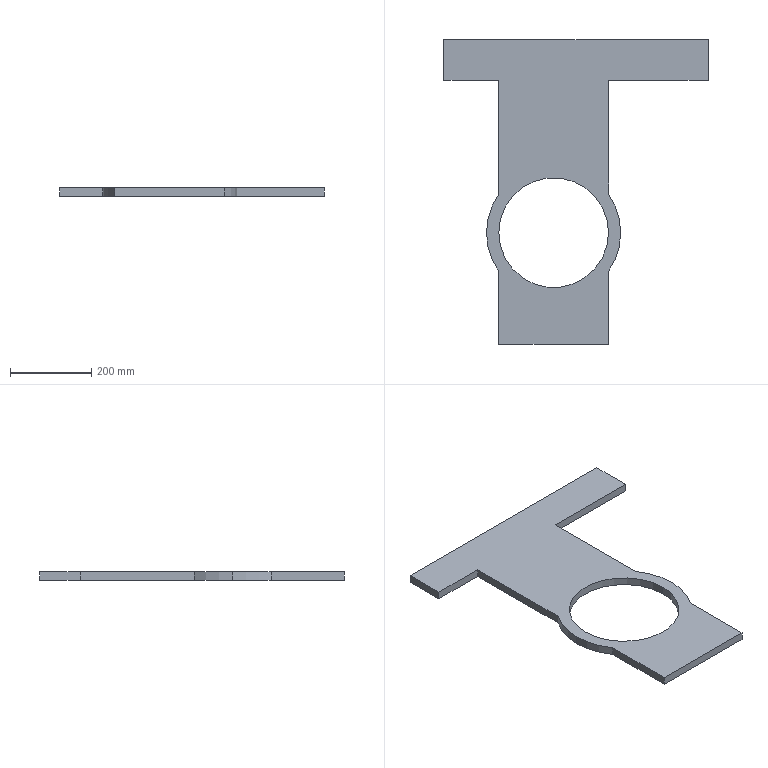Part | SolidWorks | features ICE 2, Extrusion 1 | 1 solid | 17 faces | box 650 x 750 x 20 mm | volume 3819673 mm3 | plane 12 | cylinder 5 | commonest cylinder face diameters 330 x3 270 x2
STEP:
#1=CARTESIAN_POINT('',(-135.,0.,20.));
#2=VERTEX_POINT('',#1);
#3=CARTESIAN_POINT('',(135.,0.,20.));
#4=VERTEX_POINT('',#3);
#5=CARTESIAN_POINT('',(0.,0.,20.));
#6=DIRECTION('',(0.,0.,1.));
#7=DIRECTION('',(1.,0.,0.));
#8=AXIS2_PLACEMENT_3D('',#5,#6,#7);
#9=CIRCLE('',#8,135.);
#10=EDGE_CURVE('',#2,#4,#9,.T.);
#11=ORIENTED_EDGE('',*,*,#10,.T.);
#12=CARTESIAN_POINT('',(135.,0.,0.));
#13=VERTEX_POINT('',#12);
#14=CARTESIAN_POINT('',(135.,0.,20.));
#15=DIRECTION('',(0.,0.,-1.));
#16=VECTOR('',#15,1000.);
#17=LINE('',#14,#16);
#18=EDGE_CURVE('',#4,#13,#17,.T.);
#19=ORIENTED_EDGE('',*,*,#18,.T.);
#20=CARTESIAN_POINT('',(-135.,0.,0.));
#21=VERTEX_POINT('',#20);
#22=CARTESIAN_POINT('',(0.,0.,0.));
#23=DIRECTION('',(0.,0.,1.));
#24=DIRECTION('',(1.,0.,0.));
#25=AXIS2_PLACEMENT_3D('',#22,#23,#24);
#26=CIRCLE('',#25,135.);
#27=EDGE_CURVE('',#21,#13,#26,.T.);
#28=ORIENTED_EDGE('',*,*,#27,.F.);
#29=CARTESIAN_POINT('',(-135.,0.,20.));
#30=DIRECTION('',(0.,0.,-1.));
#31=VECTOR('',#30,1000.);
#32=LINE('',#29,#31);
#33=EDGE_CURVE('',#2,#21,#32,.T.);
#34=ORIENTED_EDGE('',*,*,#33,.F.);
#35=EDGE_LOOP('',(#11,#19,#28,#34));
#36=FACE_OUTER_BOUND('',#35,.T.);
#37=CARTESIAN_POINT('',(0.,0.,20.));
#38=DIRECTION('',(0.,0.,-1.));
#39=DIRECTION('',(-1.,0.,0.));
#40=AXIS2_PLACEMENT_3D('',#37,#38,#39);
#41=CYLINDRICAL_SURFACE('',#40,135.);
#42=ADVANCED_FACE('',(#36),#41,.F.);
#43=CARTESIAN_POINT('',(-165.,0.,20.));
#44=VERTEX_POINT('',#43);
#45=CARTESIAN_POINT('',(-135.,-94.868,20.));
#46=VERTEX_POINT('',#45);
#47=CARTESIAN_POINT('',(0.,0.,20.));
#48=DIRECTION('',(0.,0.,1.));
#49=DIRECTION('',(1.,0.,0.));
#50=AXIS2_PLACEMENT_3D('',#47,#48,#49);
#51=CIRCLE('',#50,165.);
#52=EDGE_CURVE('',#44,#46,#51,.T.);
#53=ORIENTED_EDGE('',*,*,#52,.F.);
#54=CARTESIAN_POINT('',(-165.,0.,0.));
#55=VERTEX_POINT('',#54);
#56=CARTESIAN_POINT('',(-165.,0.,20.));
#57=DIRECTION('',(0.,0.,-1.));
#58=VECTOR('',#57,1000.);
#59=LINE('',#56,#58);
#60=EDGE_CURVE('',#44,#55,#59,.T.);
#61=ORIENTED_EDGE('',*,*,#60,.T.);
#62=CARTESIAN_POINT('',(-135.,-94.868,0.));
#63=VERTEX_POINT('',#62);
#64=CARTESIAN_POINT('',(0.,0.,0.));
#65=DIRECTION('',(0.,0.,1.));
#66=DIRECTION('',(1.,0.,0.));
#67=AXIS2_PLACEMENT_3D('',#64,#65,#66);
#68=CIRCLE('',#67,165.);
#69=EDGE_CURVE('',#55,#63,#68,.T.);
#70=ORIENTED_EDGE('',*,*,#69,.T.);
#71=CARTESIAN_POINT('',(-135.,-94.868,20.));
#72=DIRECTION('',(0.,0.,-1.));
#73=VECTOR('',#72,1000.);
#74=LINE('',#71,#73);
#75=EDGE_CURVE('',#46,#63,#74,.T.);
#76=ORIENTED_EDGE('',*,*,#75,.F.);
#77=EDGE_LOOP('',(#53,#61,#70,#76));
#78=FACE_OUTER_BOUND('',#77,.T.);
#79=CARTESIAN_POINT('',(0.,0.,20.));
#80=DIRECTION('',(0.,0.,-1.));
#81=DIRECTION('',(-1.,0.,0.));
#82=AXIS2_PLACEMENT_3D('',#79,#80,#81);
#83=CYLINDRICAL_SURFACE('',#82,165.);
#84=ADVANCED_FACE('',(#78),#83,.T.);
#85=CARTESIAN_POINT('',(135.,375.,20.));
#86=VERTEX_POINT('',#85);
#87=CARTESIAN_POINT('',(135.,375.,0.));
#88=VERTEX_POINT('',#87);
#89=CARTESIAN_POINT('',(135.,375.,20.));
#90=DIRECTION('',(0.,0.,-1.));
#91=VECTOR('',#90,1000.);
#92=LINE('',#89,#91);
#93=EDGE_CURVE('',#86,#88,#92,.T.);
#94=ORIENTED_EDGE('',*,*,#93,.F.);
#95=CARTESIAN_POINT('',(135.,94.868,20.));
#96=VERTEX_POINT('',#95);
#97=CARTESIAN_POINT('',(135.,475.,20.));
#98=DIRECTION('',(0.,1.,0.));
#99=VECTOR('',#98,1000.);
#100=LINE('',#97,#99);
#101=EDGE_CURVE('',#96,#86,#100,.T.);
#102=ORIENTED_EDGE('',*,*,#101,.F.);
#103=CARTESIAN_POINT('',(135.,94.868,0.));
#104=VERTEX_POINT('',#103);
#105=CARTESIAN_POINT('',(135.,94.868,20.));
#106=DIRECTION('',(0.,0.,-1.));
#107=VECTOR('',#106,1000.);
#108=LINE('',#105,#107);
#109=EDGE_CURVE('',#96,#104,#108,.T.);
#110=ORIENTED_EDGE('',*,*,#109,.T.);
#111=CARTESIAN_POINT('',(135.,475.,0.));
#112=DIRECTION('',(0.,1.,0.));
#113=VECTOR('',#112,1000.);
#114=LINE('',#111,#113);
#115=EDGE_CURVE('',#104,#88,#114,.T.);
#116=ORIENTED_EDGE('',*,*,#115,.T.);
#117=EDGE_LOOP('',(#94,#102,#110,#116));
#118=FACE_OUTER_BOUND('',#117,.T.);
#119=CARTESIAN_POINT('',(135.,475.,20.));
#120=DIRECTION('',(-1.,0.,0.));
#121=DIRECTION('',(0.,-1.,0.));
#122=AXIS2_PLACEMENT_3D('',#119,#120,#121);
#123=PLANE('',#122);
#124=ADVANCED_FACE('',(#118),#123,.F.);
#125=CARTESIAN_POINT('',(135.,-275.,20.));
#126=VERTEX_POINT('',#125);
#127=CARTESIAN_POINT('',(-135.,-275.,20.));
#128=VERTEX_POINT('',#127);
#129=CARTESIAN_POINT('',(135.,-275.,20.));
#130=DIRECTION('',(-1.,0.,0.));
#131=VECTOR('',#130,1000.);
#132=LINE('',#129,#131);
#133=EDGE_CURVE('',#126,#128,#132,.T.);
#134=ORIENTED_EDGE('',*,*,#133,.F.);
#135=CARTESIAN_POINT('',(135.,-94.868,20.));
#136=VERTEX_POINT('',#135);
#137=CARTESIAN_POINT('',(135.,-475.,20.));
#138=DIRECTION('',(0.,1.,0.));
#139=VECTOR('',#138,1000.);
#140=LINE('',#137,#139);
#141=EDGE_CURVE('',#126,#136,#140,.T.);
#142=ORIENTED_EDGE('',*,*,#141,.T.);
#143=CARTESIAN_POINT('',(0.,0.,20.));
#144=DIRECTION('',(0.,0.,1.));
#145=DIRECTION('',(1.,0.,0.));
#146=AXIS2_PLACEMENT_3D('',#143,#144,#145);
#147=CIRCLE('',#146,165.);
#148=EDGE_CURVE('',#136,#96,#147,.T.);
#149=ORIENTED_EDGE('',*,*,#148,.T.);
#150=ORIENTED_EDGE('',*,*,#101,.T.);
#151=CARTESIAN_POINT('',(380.,375.,20.));
#152=VERTEX_POINT('',#151);
#153=CARTESIAN_POINT('',(0.,375.,20.));
#154=DIRECTION('',(1.,0.,0.));
#155=VECTOR('',#154,1000.);
#156=LINE('',#153,#155);
#157=EDGE_CURVE('',#86,#152,#156,.T.);
#158=ORIENTED_EDGE('',*,*,#157,.T.);
#159=CARTESIAN_POINT('',(380.,475.,20.));
#160=VERTEX_POINT('',#159);
#161=CARTESIAN_POINT('',(380.,0.,20.));
#162=DIRECTION('',(0.,-1.,0.));
#163=VECTOR('',#162,1000.);
#164=LINE('',#161,#163);
#165=EDGE_CURVE('',#160,#152,#164,.T.);
#166=ORIENTED_EDGE('',*,*,#165,.F.);
#167=CARTESIAN_POINT('',(-270.,475.,20.));
#168=VERTEX_POINT('',#167);
#169=CARTESIAN_POINT('',(135.,475.,20.));
#170=DIRECTION('',(-1.,0.,0.));
#171=VECTOR('',#170,1000.);
#172=LINE('',#169,#171);
#173=EDGE_CURVE('',#160,#168,#172,.T.);
#174=ORIENTED_EDGE('',*,*,#173,.T.);
#175=CARTESIAN_POINT('',(-270.,375.,20.));
#176=VERTEX_POINT('',#175);
#177=CARTESIAN_POINT('',(-270.,0.,20.));
#178=DIRECTION('',(0.,-1.,0.));
#179=VECTOR('',#178,1000.);
#180=LINE('',#177,#179);
#181=EDGE_CURVE('',#168,#176,#180,.T.);
#182=ORIENTED_EDGE('',*,*,#181,.T.);
#183=CARTESIAN_POINT('',(-135.,375.,20.));
#184=VERTEX_POINT('',#183);
#185=CARTESIAN_POINT('',(0.,375.,20.));
#186=DIRECTION('',(-1.,0.,0.));
#187=VECTOR('',#186,1000.);
#188=LINE('',#185,#187);
#189=EDGE_CURVE('',#184,#176,#188,.T.);
#190=ORIENTED_EDGE('',*,*,#189,.F.);
#191=CARTESIAN_POINT('',(-135.,94.868,20.));
#192=VERTEX_POINT('',#191);
#193=CARTESIAN_POINT('',(-135.,475.,20.));
#194=DIRECTION('',(0.,-1.,0.));
#195=VECTOR('',#194,1000.);
#196=LINE('',#193,#195);
#197=EDGE_CURVE('',#184,#192,#196,.T.);
#198=ORIENTED_EDGE('',*,*,#197,.T.);
#199=CARTESIAN_POINT('',(0.,0.,20.));
#200=DIRECTION('',(0.,0.,1.));
#201=DIRECTION('',(1.,0.,0.));
#202=AXIS2_PLACEMENT_3D('',#199,#200,#201);
#203=CIRCLE('',#202,165.);
#204=EDGE_CURVE('',#192,#44,#203,.T.);
#205=ORIENTED_EDGE('',*,*,#204,.T.);
#206=ORIENTED_EDGE('',*,*,#52,.T.);
#207=CARTESIAN_POINT('',(-135.,-475.,20.));
#208=DIRECTION('',(0.,-1.,0.));
#209=VECTOR('',#208,1000.);
#210=LINE('',#207,#209);
#211=EDGE_CURVE('',#46,#128,#210,.T.);
#212=ORIENTED_EDGE('',*,*,#211,.T.);
#213=EDGE_LOOP('',(#134,#142,#149,#150,#158,#166,#174,#182,#190,#198,#205,#206,#212));
#214=FACE_OUTER_BOUND('',#213,.T.);
#215=ORIENTED_EDGE('',*,*,#10,.F.);
#216=CARTESIAN_POINT('',(0.,0.,20.));
#217=DIRECTION('',(0.,0.,1.));
#218=DIRECTION('',(1.,0.,0.));
#219=AXIS2_PLACEMENT_3D('',#216,#217,#218);
#220=CIRCLE('',#219,135.);
#221=EDGE_CURVE('',#4,#2,#220,.T.);
#222=ORIENTED_EDGE('',*,*,#221,.F.);
#223=EDGE_LOOP('',(#215,#222));
#224=FACE_BOUND('',#223,.T.);
#225=CARTESIAN_POINT('',(0.,0.,20.));
#226=DIRECTION('',(0.,0.,1.));
#227=DIRECTION('',(1.,0.,0.));
#228=AXIS2_PLACEMENT_3D('',#225,#226,#227);
#229=PLANE('',#228);
#230=ADVANCED_FACE('',(#214,#224),#229,.T.);
#231=CARTESIAN_POINT('',(135.,-275.,0.));
#232=VERTEX_POINT('',#231);
#233=CARTESIAN_POINT('',(135.,-94.868,0.));
#234=VERTEX_POINT('',#233);
#235=CARTESIAN_POINT('',(135.,-475.,0.));
#236=DIRECTION('',(0.,1.,0.));
#237=VECTOR('',#236,1000.);
#238=LINE('',#235,#237);
#239=EDGE_CURVE('',#232,#234,#238,.T.);
#240=ORIENTED_EDGE('',*,*,#239,.F.);
#241=CARTESIAN_POINT('',(-135.,-275.,0.));
#242=VERTEX_POINT('',#241);
#243=CARTESIAN_POINT('',(135.,-275.,0.));
#244=DIRECTION('',(-1.,0.,0.));
#245=VECTOR('',#244,1000.);
#246=LINE('',#243,#245);
#247=EDGE_CURVE('',#232,#242,#246,.T.);
#248=ORIENTED_EDGE('',*,*,#247,.T.);
#249=CARTESIAN_POINT('',(-135.,-475.,0.));
#250=DIRECTION('',(0.,-1.,0.));
#251=VECTOR('',#250,1000.);
#252=LINE('',#249,#251);
#253=EDGE_CURVE('',#63,#242,#252,.T.);
#254=ORIENTED_EDGE('',*,*,#253,.F.);
#255=ORIENTED_EDGE('',*,*,#69,.F.);
#256=CARTESIAN_POINT('',(-135.,94.868,0.));
#257=VERTEX_POINT('',#256);
#258=CARTESIAN_POINT('',(0.,0.,0.));
#259=DIRECTION('',(0.,0.,1.));
#260=DIRECTION('',(1.,0.,0.));
#261=AXIS2_PLACEMENT_3D('',#258,#259,#260);
#262=CIRCLE('',#261,165.);
#263=EDGE_CURVE('',#257,#55,#262,.T.);
#264=ORIENTED_EDGE('',*,*,#263,.F.);
#265=CARTESIAN_POINT('',(-135.,375.,0.));
#266=VERTEX_POINT('',#265);
#267=CARTESIAN_POINT('',(-135.,475.,0.));
#268=DIRECTION('',(0.,-1.,0.));
#269=VECTOR('',#268,1000.);
#270=LINE('',#267,#269);
#271=EDGE_CURVE('',#266,#257,#270,.T.);
#272=ORIENTED_EDGE('',*,*,#271,.F.);
#273=CARTESIAN_POINT('',(-270.,375.,0.));
#274=VERTEX_POINT('',#273);
#275=CARTESIAN_POINT('',(0.,375.,0.));
#276=DIRECTION('',(-1.,0.,0.));
#277=VECTOR('',#276,1000.);
#278=LINE('',#275,#277);
#279=EDGE_CURVE('',#266,#274,#278,.T.);
#280=ORIENTED_EDGE('',*,*,#279,.T.);
#281=CARTESIAN_POINT('',(-270.,475.,0.));
#282=VERTEX_POINT('',#281);
#283=CARTESIAN_POINT('',(-270.,0.,0.));
#284=DIRECTION('',(0.,-1.,0.));
#285=VECTOR('',#284,1000.);
#286=LINE('',#283,#285);
#287=EDGE_CURVE('',#282,#274,#286,.T.);
#288=ORIENTED_EDGE('',*,*,#287,.F.);
#289=CARTESIAN_POINT('',(380.,475.,0.));
#290=VERTEX_POINT('',#289);
#291=CARTESIAN_POINT('',(135.,475.,0.));
#292=DIRECTION('',(-1.,0.,0.));
#293=VECTOR('',#292,1000.);
#294=LINE('',#291,#293);
#295=EDGE_CURVE('',#290,#282,#294,.T.);
#296=ORIENTED_EDGE('',*,*,#295,.F.);
#297=CARTESIAN_POINT('',(380.,375.,0.));
#298=VERTEX_POINT('',#297);
#299=CARTESIAN_POINT('',(380.,0.,0.));
#300=DIRECTION('',(0.,-1.,0.));
#301=VECTOR('',#300,1000.);
#302=LINE('',#299,#301);
#303=EDGE_CURVE('',#290,#298,#302,.T.);
#304=ORIENTED_EDGE('',*,*,#303,.T.);
#305=CARTESIAN_POINT('',(0.,375.,0.));
#306=DIRECTION('',(1.,0.,0.));
#307=VECTOR('',#306,1000.);
#308=LINE('',#305,#307);
#309=EDGE_CURVE('',#88,#298,#308,.T.);
#310=ORIENTED_EDGE('',*,*,#309,.F.);
#311=ORIENTED_EDGE('',*,*,#115,.F.);
#312=CARTESIAN_POINT('',(0.,0.,0.));
#313=DIRECTION('',(0.,0.,1.));
#314=DIRECTION('',(1.,0.,0.));
#315=AXIS2_PLACEMENT_3D('',#312,#313,#314);
#316=CIRCLE('',#315,165.);
#317=EDGE_CURVE('',#234,#104,#316,.T.);
#318=ORIENTED_EDGE('',*,*,#317,.F.);
#319=EDGE_LOOP('',(#240,#248,#254,#255,#264,#272,#280,#288,#296,#304,#310,#311,#318));
#320=FACE_OUTER_BOUND('',#319,.T.);
#321=ORIENTED_EDGE('',*,*,#27,.T.);
#322=CARTESIAN_POINT('',(0.,0.,0.));
#323=DIRECTION('',(0.,0.,1.));
#324=DIRECTION('',(1.,0.,0.));
#325=AXIS2_PLACEMENT_3D('',#322,#323,#324);
#326=CIRCLE('',#325,135.);
#327=EDGE_CURVE('',#13,#21,#326,.T.);
#328=ORIENTED_EDGE('',*,*,#327,.T.);
#329=EDGE_LOOP('',(#321,#328));
#330=FACE_BOUND('',#329,.T.);
#331=CARTESIAN_POINT('',(0.,0.,0.));
#332=DIRECTION('',(0.,0.,1.));
#333=DIRECTION('',(1.,0.,0.));
#334=AXIS2_PLACEMENT_3D('',#331,#332,#333);
#335=PLANE('',#334);
#336=ADVANCED_FACE('',(#320,#330),#335,.F.);
#337=ORIENTED_EDGE('',*,*,#295,.T.);
#338=CARTESIAN_POINT('',(-270.,475.,20.));
#339=DIRECTION('',(0.,0.,-1.));
#340=VECTOR('',#339,1000.);
#341=LINE('',#338,#340);
#342=EDGE_CURVE('',#168,#282,#341,.T.);
#343=ORIENTED_EDGE('',*,*,#342,.F.);
#344=ORIENTED_EDGE('',*,*,#173,.F.);
#345=CARTESIAN_POINT('',(380.,475.,20.));
#346=DIRECTION('',(0.,0.,-1.));
#347=VECTOR('',#346,1000.);
#348=LINE('',#345,#347);
#349=EDGE_CURVE('',#160,#290,#348,.T.);
#350=ORIENTED_EDGE('',*,*,#349,.T.);
#351=EDGE_LOOP('',(#337,#343,#344,#350));
#352=FACE_OUTER_BOUND('',#351,.T.);
#353=CARTESIAN_POINT('',(135.,475.,20.));
#354=DIRECTION('',(0.,-1.,0.));
#355=DIRECTION('',(1.,0.,0.));
#356=AXIS2_PLACEMENT_3D('',#353,#354,#355);
#357=PLANE('',#356);
#358=ADVANCED_FACE('',(#352),#357,.F.);
#359=ORIENTED_EDGE('',*,*,#197,.F.);
#360=CARTESIAN_POINT('',(-135.,375.,20.));
#361=DIRECTION('',(0.,0.,-1.));
#362=VECTOR('',#361,1000.);
#363=LINE('',#360,#362);
#364=EDGE_CURVE('',#184,#266,#363,.T.);
#365=ORIENTED_EDGE('',*,*,#364,.T.);
#366=ORIENTED_EDGE('',*,*,#271,.T.);
#367=CARTESIAN_POINT('',(-135.,94.868,20.));
#368=DIRECTION('',(0.,0.,-1.));
#369=VECTOR('',#368,1000.);
#370=LINE('',#367,#369);
#371=EDGE_CURVE('',#192,#257,#370,.T.);
#372=ORIENTED_EDGE('',*,*,#371,.F.);
#373=EDGE_LOOP('',(#359,#365,#366,#372));
#374=FACE_OUTER_BOUND('',#373,.T.);
#375=CARTESIAN_POINT('',(-135.,475.,20.));
#376=DIRECTION('',(1.,0.,0.));
#377=DIRECTION('',(0.,1.,0.));
#378=AXIS2_PLACEMENT_3D('',#375,#376,#377);
#379=PLANE('',#378);
#380=ADVANCED_FACE('',(#374),#379,.F.);
#381=ORIENTED_EDGE('',*,*,#60,.F.);
#382=ORIENTED_EDGE('',*,*,#204,.F.);
#383=ORIENTED_EDGE('',*,*,#371,.T.);
#384=ORIENTED_EDGE('',*,*,#263,.T.);
#385=EDGE_LOOP('',(#381,#382,#383,#384));
#386=FACE_OUTER_BOUND('',#385,.T.);
#387=CARTESIAN_POINT('',(0.,0.,20.));
#388=DIRECTION('',(0.,0.,-1.));
#389=DIRECTION('',(-1.,0.,0.));
#390=AXIS2_PLACEMENT_3D('',#387,#388,#389);
#391=CYLINDRICAL_SURFACE('',#390,165.);
#392=ADVANCED_FACE('',(#386),#391,.T.);
#393=ORIENTED_EDGE('',*,*,#253,.T.);
#394=CARTESIAN_POINT('',(-135.,-275.,0.));
#395=DIRECTION('',(0.,0.,1.));
#396=VECTOR('',#395,1000.);
#397=LINE('',#394,#396);
#398=EDGE_CURVE('',#242,#128,#397,.T.);
#399=ORIENTED_EDGE('',*,*,#398,.T.);
#400=ORIENTED_EDGE('',*,*,#211,.F.);
#401=ORIENTED_EDGE('',*,*,#75,.T.);
#402=EDGE_LOOP('',(#393,#399,#400,#401));
#403=FACE_OUTER_BOUND('',#402,.T.);
#404=CARTESIAN_POINT('',(-135.,-475.,20.));
#405=DIRECTION('',(1.,0.,0.));
#406=DIRECTION('',(0.,1.,0.));
#407=AXIS2_PLACEMENT_3D('',#404,#405,#406);
#408=PLANE('',#407);
#409=ADVANCED_FACE('',(#403),#408,.F.);
#410=ORIENTED_EDGE('',*,*,#141,.F.);
#411=CARTESIAN_POINT('',(135.,-275.,0.));
#412=DIRECTION('',(0.,0.,1.));
#413=VECTOR('',#412,1000.);
#414=LINE('',#411,#413);
#415=EDGE_CURVE('',#232,#126,#414,.T.);
#416=ORIENTED_EDGE('',*,*,#415,.F.);
#417=ORIENTED_EDGE('',*,*,#239,.T.);
#418=CARTESIAN_POINT('',(135.,-94.868,20.));
#419=DIRECTION('',(0.,0.,-1.));
#420=VECTOR('',#419,1000.);
#421=LINE('',#418,#420);
#422=EDGE_CURVE('',#136,#234,#421,.T.);
#423=ORIENTED_EDGE('',*,*,#422,.F.);
#424=EDGE_LOOP('',(#410,#416,#417,#423));
#425=FACE_OUTER_BOUND('',#424,.T.);
#426=CARTESIAN_POINT('',(135.,-475.,20.));
#427=DIRECTION('',(-1.,0.,0.));
#428=DIRECTION('',(0.,-1.,0.));
#429=AXIS2_PLACEMENT_3D('',#426,#427,#428);
#430=PLANE('',#429);
#431=ADVANCED_FACE('',(#425),#430,.F.);
#432=ORIENTED_EDGE('',*,*,#317,.T.);
#433=ORIENTED_EDGE('',*,*,#109,.F.);
#434=ORIENTED_EDGE('',*,*,#148,.F.);
#435=ORIENTED_EDGE('',*,*,#422,.T.);
#436=EDGE_LOOP('',(#432,#433,#434,#435));
#437=FACE_OUTER_BOUND('',#436,.T.);
#438=CARTESIAN_POINT('',(0.,0.,20.));
#439=DIRECTION('',(0.,0.,-1.));
#440=DIRECTION('',(-1.,0.,0.));
#441=AXIS2_PLACEMENT_3D('',#438,#439,#440);
#442=CYLINDRICAL_SURFACE('',#441,165.);
#443=ADVANCED_FACE('',(#437),#442,.T.);
#444=ORIENTED_EDGE('',*,*,#18,.F.);
#445=ORIENTED_EDGE('',*,*,#221,.T.);
#446=ORIENTED_EDGE('',*,*,#33,.T.);
#447=ORIENTED_EDGE('',*,*,#327,.F.);
#448=EDGE_LOOP('',(#444,#445,#446,#447));
#449=FACE_OUTER_BOUND('',#448,.T.);
#450=CARTESIAN_POINT('',(0.,0.,20.));
#451=DIRECTION('',(0.,0.,-1.));
#452=DIRECTION('',(-1.,0.,0.));
#453=AXIS2_PLACEMENT_3D('',#450,#451,#452);
#454=CYLINDRICAL_SURFACE('',#453,135.);
#455=ADVANCED_FACE('',(#449),#454,.F.);
#456=ORIENTED_EDGE('',*,*,#133,.T.);
#457=ORIENTED_EDGE('',*,*,#398,.F.);
#458=ORIENTED_EDGE('',*,*,#247,.F.);
#459=ORIENTED_EDGE('',*,*,#415,.T.);
#460=EDGE_LOOP('',(#456,#457,#458,#459));
#461=FACE_OUTER_BOUND('',#460,.T.);
#462=CARTESIAN_POINT('',(135.,-275.,0.));
#463=DIRECTION('',(0.,1.,0.));
#464=DIRECTION('',(-1.,0.,0.));
#465=AXIS2_PLACEMENT_3D('',#462,#463,#464);
#466=PLANE('',#465);
#467=ADVANCED_FACE('',(#461),#466,.F.);
#468=ORIENTED_EDGE('',*,*,#309,.T.);
#469=CARTESIAN_POINT('',(380.,375.,20.));
#470=DIRECTION('',(0.,0.,-1.));
#471=VECTOR('',#470,1000.);
#472=LINE('',#469,#471);
#473=EDGE_CURVE('',#152,#298,#472,.T.);
#474=ORIENTED_EDGE('',*,*,#473,.F.);
#475=ORIENTED_EDGE('',*,*,#157,.F.);
#476=ORIENTED_EDGE('',*,*,#93,.T.);
#477=EDGE_LOOP('',(#468,#474,#475,#476));
#478=FACE_OUTER_BOUND('',#477,.T.);
#479=CARTESIAN_POINT('',(0.,375.,20.));
#480=DIRECTION('',(0.,1.,0.));
#481=DIRECTION('',(-1.,0.,0.));
#482=AXIS2_PLACEMENT_3D('',#479,#480,#481);
#483=PLANE('',#482);
#484=ADVANCED_FACE('',(#478),#483,.F.);
#485=ORIENTED_EDGE('',*,*,#303,.F.);
#486=ORIENTED_EDGE('',*,*,#349,.F.);
#487=ORIENTED_EDGE('',*,*,#165,.T.);
#488=ORIENTED_EDGE('',*,*,#473,.T.);
#489=EDGE_LOOP('',(#485,#486,#487,#488));
#490=FACE_OUTER_BOUND('',#489,.T.);
#491=CARTESIAN_POINT('',(380.,0.,20.));
#492=DIRECTION('',(1.,0.,0.));
#493=DIRECTION('',(0.,1.,0.));
#494=AXIS2_PLACEMENT_3D('',#491,#492,#493);
#495=PLANE('',#494);
#496=ADVANCED_FACE('',(#490),#495,.T.);
#497=ORIENTED_EDGE('',*,*,#287,.T.);
#498=CARTESIAN_POINT('',(-270.,375.,20.));
#499=DIRECTION('',(0.,0.,-1.));
#500=VECTOR('',#499,1000.);
#501=LINE('',#498,#500);
#502=EDGE_CURVE('',#176,#274,#501,.T.);
#503=ORIENTED_EDGE('',*,*,#502,.F.);
#504=ORIENTED_EDGE('',*,*,#181,.F.);
#505=ORIENTED_EDGE('',*,*,#342,.T.);
#506=EDGE_LOOP('',(#497,#503,#504,#505));
#507=FACE_OUTER_BOUND('',#506,.T.);
#508=CARTESIAN_POINT('',(-270.,0.,20.));
#509=DIRECTION('',(1.,0.,0.));
#510=DIRECTION('',(0.,0.,-1.));
#511=AXIS2_PLACEMENT_3D('',#508,#509,#510);
#512=PLANE('',#511);
#513=ADVANCED_FACE('',(#507),#512,.F.);
#514=ORIENTED_EDGE('',*,*,#279,.F.);
#515=ORIENTED_EDGE('',*,*,#364,.F.);
#516=ORIENTED_EDGE('',*,*,#189,.T.);
#517=ORIENTED_EDGE('',*,*,#502,.T.);
#518=EDGE_LOOP('',(#514,#515,#516,#517));
#519=FACE_OUTER_BOUND('',#518,.T.);
#520=CARTESIAN_POINT('',(0.,375.,20.));
#521=DIRECTION('',(0.,-1.,0.));
#522=DIRECTION('',(0.,0.,-1.));
#523=AXIS2_PLACEMENT_3D('',#520,#521,#522);
#524=PLANE('',#523);
#525=ADVANCED_FACE('',(#519),#524,.T.);
#526=CLOSED_SHELL('',(#42,#84,#124,#230,#336,#358,#380,#392,#409,#431,#443,#455,#467,#484,#496,#513,#525));
#527=MANIFOLD_SOLID_BREP('',#526);
#528=CARTESIAN_POINT('',(0.,0.,0.));
#529=DIRECTION('',(0.,0.,1.));
#530=DIRECTION('',(1.,0.,0.));
#531=AXIS2_PLACEMENT_3D('',#528,#529,#530);
#532=(LENGTH_UNIT()NAMED_UNIT(*)SI_UNIT(.MILLI.,.METRE.));
#533=UNCERTAINTY_MEASURE_WITH_UNIT(LENGTH_MEASURE(0.00001),#532,'','');
#534=(NAMED_UNIT(*)PLANE_ANGLE_UNIT()SI_UNIT($,.RADIAN.));
#535=(NAMED_UNIT(*)SI_UNIT($,.STERADIAN.)SOLID_ANGLE_UNIT());
#536=(GEOMETRIC_REPRESENTATION_CONTEXT(3)GLOBAL_UNCERTAINTY_ASSIGNED_CONTEXT((#533))GLOBAL_UNIT_ASSIGNED_CONTEXT((#532,#534,#535))REPRESENTATION_CONTEXT('',''));
#537=ADVANCED_BREP_SHAPE_REPRESENTATION('',(#527,#531),#536);